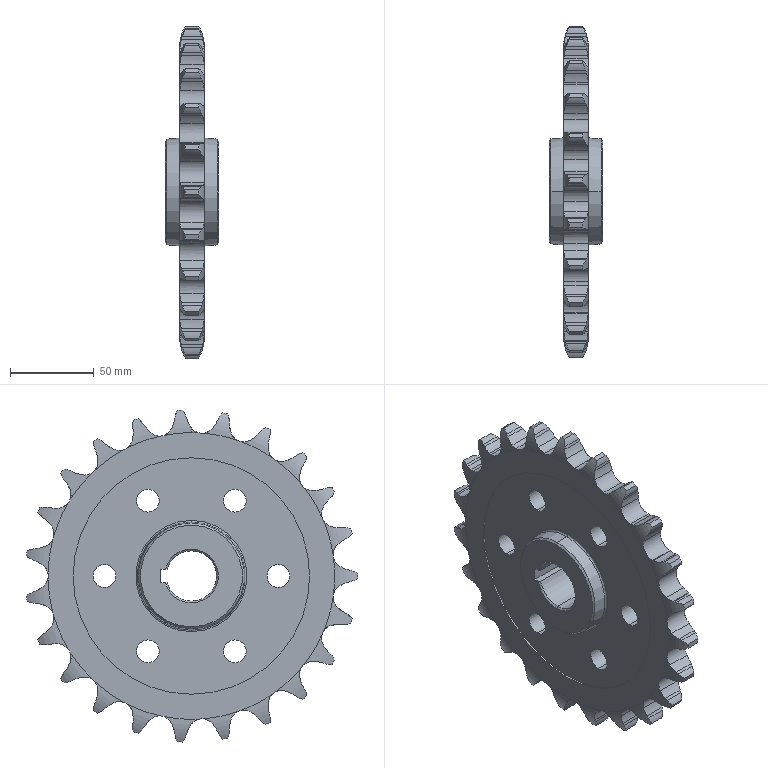Part | SolidWorks | features Cut 3, CirPattern 2, Revolution 2, Chamfer 1, Fillet 1, MirrorPattern 1 | 1 solid | 290 faces | box 32 x 197.271 x 197.721 mm | volume 369448 mm3 | cylinder 169 | plane 55 | torus 52 | cone 14 | commonest cylinder face diameters 23.032 x49 41.467 x48 16.059 x30 198 x23 13.533 x12 140.816 x4